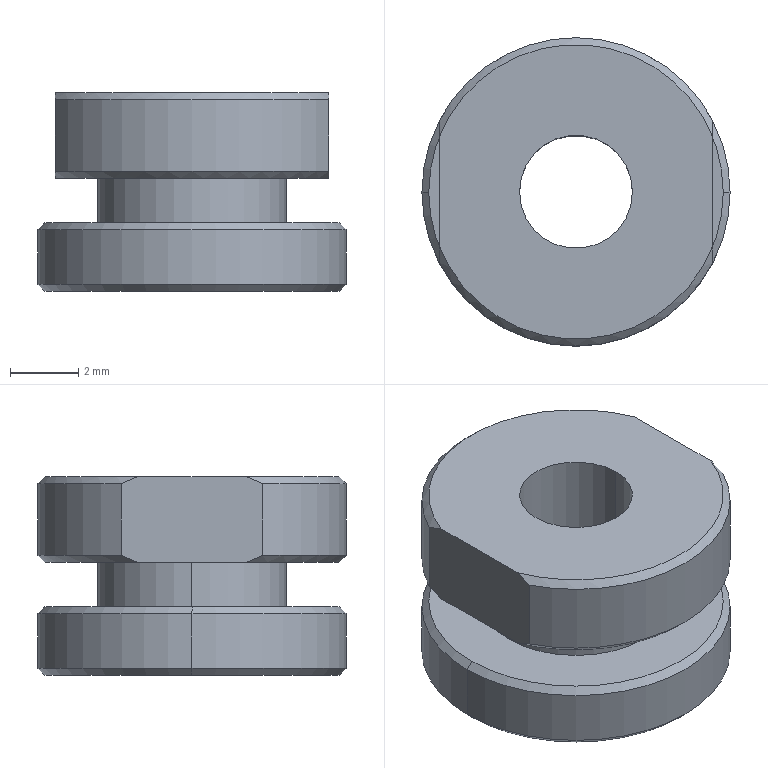Part | STEP file | 1 solid | 22 faces | box 9 x 9 x 5.8 mm | volume 258.691 mm3 | cone 8 | cylinder 8 | plane 6 | commonest cylinder face diameters 9 x4 3.3 x2 5.5 x2